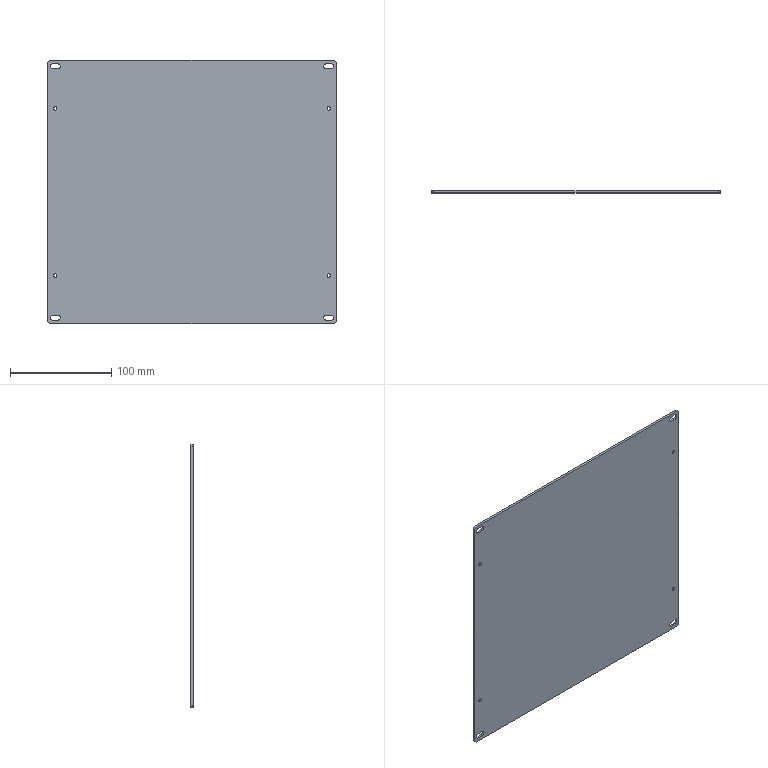Part | STEP file | 227H056376 BKT_Default | 1 solid | 34 faces | box 285 x 2 x 260 mm | volume 147758 mm3 | plane 18 | cylinder 16 | commonest cylinder face diameters 3.3 x8 5 x8